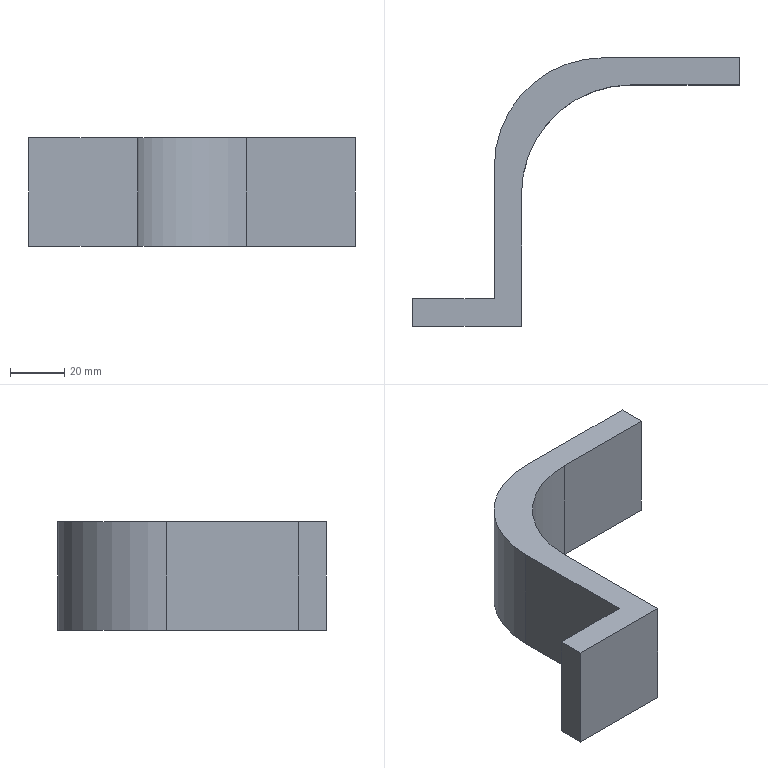Part | STEP file | Pressure Rod | 1 solid | 12 faces | box 120 x 98.5 x 40 mm | volume 83400 mm3 | plane 10 | cylinder 2 | commonest cylinder face diameters 80 x2
STEP:
#1=CARTESIAN_POINT('',(0.,0.,0.));
#2=DIRECTION('',(0.,0.,1.));
#3=DIRECTION('',(1.,0.,0.));
#4=AXIS2_PLACEMENT_3D('',#1,#2,#3);
#5=CARTESIAN_POINT('',(0.,-10.,-20.));
#6=VERTEX_POINT('',#5);
#7=CARTESIAN_POINT('',(0.,0.,-20.));
#8=VERTEX_POINT('',#7);
#9=CARTESIAN_POINT('',(0.,-10.,-20.));
#10=DIRECTION('',(0.,1.,0.));
#11=VECTOR('',#10,1.);
#12=LINE('',#9,#11);
#13=CARTESIAN_POINT('',(0.,-10.,20.));
#14=DIRECTION('',(-1.,0.,0.));
#15=DIRECTION('',(0.,0.,1.));
#16=AXIS2_PLACEMENT_3D('',#13,#14,#15);
#17=PLANE('',#16);
#18=CARTESIAN_POINT('',(-40.,0.));
#19=DIRECTION('',(0.,1.));
#20=VECTOR('',#19,1.);
#21=LINE('',#18,#20);
#22=(GEOMETRIC_REPRESENTATION_CONTEXT(2)PARAMETRIC_REPRESENTATION_CONTEXT()REPRESENTATION_CONTEXT('',''));
#23=DEFINITIONAL_REPRESENTATION('',(#21),#22);
#24=PCURVE('',#17,#23);
#25=CARTESIAN_POINT('',(0.,0.,-20.));
#26=DIRECTION('',(0.,0.,1.));
#27=DIRECTION('',(1.,0.,0.));
#28=AXIS2_PLACEMENT_3D('',#25,#26,#27);
#29=PLANE('',#28);
#30=CARTESIAN_POINT('',(0.,-10.));
#31=DIRECTION('',(0.,1.));
#32=VECTOR('',#31,1.);
#33=LINE('',#30,#32);
#34=(GEOMETRIC_REPRESENTATION_CONTEXT(2)PARAMETRIC_REPRESENTATION_CONTEXT()REPRESENTATION_CONTEXT('',''));
#35=DEFINITIONAL_REPRESENTATION('',(#33),#34);
#36=PCURVE('',#29,#35);
#37=SURFACE_CURVE('',#12,(#24,#36),.PCURVE_S1.);
#38=EDGE_CURVE('',#6,#8,#37,.T.);
#39=ORIENTED_EDGE('',*,*,#38,.T.);
#40=CARTESIAN_POINT('',(0.,0.,20.));
#41=VERTEX_POINT('',#40);
#42=CARTESIAN_POINT('',(0.,0.,20.));
#43=DIRECTION('',(0.,0.,-1.));
#44=VECTOR('',#43,1.);
#45=LINE('',#42,#44);
#46=CARTESIAN_POINT('',(0.,10.));
#47=DIRECTION('',(-1.,0.));
#48=VECTOR('',#47,1.);
#49=LINE('',#46,#48);
#50=(GEOMETRIC_REPRESENTATION_CONTEXT(2)PARAMETRIC_REPRESENTATION_CONTEXT()REPRESENTATION_CONTEXT('',''));
#51=DEFINITIONAL_REPRESENTATION('',(#49),#50);
#52=PCURVE('',#17,#51);
#53=CARTESIAN_POINT('',(0.,0.,20.));
#54=DIRECTION('',(0.,-1.,0.));
#55=DIRECTION('',(1.,0.,0.));
#56=AXIS2_PLACEMENT_3D('',#53,#54,#55);
#57=PLANE('',#56);
#58=CARTESIAN_POINT('',(0.,0.));
#59=DIRECTION('',(0.,-1.));
#60=VECTOR('',#59,1.);
#61=LINE('',#58,#60);
#62=(GEOMETRIC_REPRESENTATION_CONTEXT(2)PARAMETRIC_REPRESENTATION_CONTEXT()REPRESENTATION_CONTEXT('',''));
#63=DEFINITIONAL_REPRESENTATION('',(#61),#62);
#64=PCURVE('',#57,#63);
#65=SURFACE_CURVE('',#45,(#52,#64),.PCURVE_S1.);
#66=EDGE_CURVE('',#41,#8,#65,.T.);
#67=ORIENTED_EDGE('',*,*,#66,.F.);
#68=CARTESIAN_POINT('',(0.,-10.,20.));
#69=VERTEX_POINT('',#68);
#70=CARTESIAN_POINT('',(0.,-10.,20.));
#71=DIRECTION('',(0.,1.,0.));
#72=VECTOR('',#71,1.);
#73=LINE('',#70,#72);
#74=CARTESIAN_POINT('',(0.,0.));
#75=DIRECTION('',(0.,1.));
#76=VECTOR('',#75,1.);
#77=LINE('',#74,#76);
#78=(GEOMETRIC_REPRESENTATION_CONTEXT(2)PARAMETRIC_REPRESENTATION_CONTEXT()REPRESENTATION_CONTEXT('',''));
#79=DEFINITIONAL_REPRESENTATION('',(#77),#78);
#80=PCURVE('',#17,#79);
#81=CARTESIAN_POINT('',(0.,0.,20.));
#82=DIRECTION('',(0.,0.,1.));
#83=DIRECTION('',(1.,0.,0.));
#84=AXIS2_PLACEMENT_3D('',#81,#82,#83);
#85=PLANE('',#84);
#86=CARTESIAN_POINT('',(0.,-10.));
#87=DIRECTION('',(0.,1.));
#88=VECTOR('',#87,1.);
#89=LINE('',#86,#88);
#90=(GEOMETRIC_REPRESENTATION_CONTEXT(2)PARAMETRIC_REPRESENTATION_CONTEXT()REPRESENTATION_CONTEXT('',''));
#91=DEFINITIONAL_REPRESENTATION('',(#89),#90);
#92=PCURVE('',#85,#91);
#93=SURFACE_CURVE('',#73,(#80,#92),.PCURVE_S1.);
#94=EDGE_CURVE('',#69,#41,#93,.T.);
#95=ORIENTED_EDGE('',*,*,#94,.F.);
#96=CARTESIAN_POINT('',(0.,-10.,20.));
#97=DIRECTION('',(0.,0.,-1.));
#98=VECTOR('',#97,1.);
#99=LINE('',#96,#98);
#100=CARTESIAN_POINT('',(0.,0.));
#101=DIRECTION('',(-1.,0.));
#102=VECTOR('',#101,1.);
#103=LINE('',#100,#102);
#104=(GEOMETRIC_REPRESENTATION_CONTEXT(2)PARAMETRIC_REPRESENTATION_CONTEXT()REPRESENTATION_CONTEXT('',''));
#105=DEFINITIONAL_REPRESENTATION('',(#103),#104);
#106=PCURVE('',#17,#105);
#107=CARTESIAN_POINT('',(-80.,-10.,20.));
#108=DIRECTION('',(0.,1.,0.));
#109=DIRECTION('',(0.,0.,1.));
#110=AXIS2_PLACEMENT_3D('',#107,#108,#109);
#111=PLANE('',#110);
#112=CARTESIAN_POINT('',(0.,80.));
#113=DIRECTION('',(-1.,0.));
#114=VECTOR('',#113,1.);
#115=LINE('',#112,#114);
#116=(GEOMETRIC_REPRESENTATION_CONTEXT(2)PARAMETRIC_REPRESENTATION_CONTEXT()REPRESENTATION_CONTEXT('',''));
#117=DEFINITIONAL_REPRESENTATION('',(#115),#116);
#118=PCURVE('',#111,#117);
#119=SURFACE_CURVE('',#99,(#106,#118),.PCURVE_S1.);
#120=EDGE_CURVE('',#69,#6,#119,.T.);
#121=ORIENTED_EDGE('',*,*,#120,.T.);
#122=EDGE_LOOP('',(#39,#67,#95,#121));
#123=FACE_BOUND('',#122,.T.);
#124=ADVANCED_FACE('',(#123),#17,.F.);
#125=CARTESIAN_POINT('',(-50.,0.,-20.));
#126=VERTEX_POINT('',#125);
#127=CARTESIAN_POINT('',(0.,0.,-20.));
#128=DIRECTION('',(-1.,0.,0.));
#129=VECTOR('',#128,1.);
#130=LINE('',#127,#129);
#131=CARTESIAN_POINT('',(0.,-40.));
#132=DIRECTION('',(-1.,0.));
#133=VECTOR('',#132,1.);
#134=LINE('',#131,#133);
#135=(GEOMETRIC_REPRESENTATION_CONTEXT(2)PARAMETRIC_REPRESENTATION_CONTEXT()REPRESENTATION_CONTEXT('',''));
#136=DEFINITIONAL_REPRESENTATION('',(#134),#135);
#137=PCURVE('',#57,#136);
#138=CARTESIAN_POINT('',(0.,0.));
#139=DIRECTION('',(-1.,0.));
#140=VECTOR('',#139,1.);
#141=LINE('',#138,#140);
#142=(GEOMETRIC_REPRESENTATION_CONTEXT(2)PARAMETRIC_REPRESENTATION_CONTEXT()REPRESENTATION_CONTEXT('',''));
#143=DEFINITIONAL_REPRESENTATION('',(#141),#142);
#144=PCURVE('',#29,#143);
#145=SURFACE_CURVE('',#130,(#137,#144),.PCURVE_S1.);
#146=EDGE_CURVE('',#8,#126,#145,.T.);
#147=ORIENTED_EDGE('',*,*,#146,.T.);
#148=CARTESIAN_POINT('',(-50.,0.,20.));
#149=VERTEX_POINT('',#148);
#150=CARTESIAN_POINT('',(-50.,0.,20.));
#151=DIRECTION('',(0.,0.,1.));
#152=VECTOR('',#151,1.);
#153=LINE('',#150,#152);
#154=CARTESIAN_POINT('',(-50.,0.));
#155=DIRECTION('',(0.,1.));
#156=VECTOR('',#155,1.);
#157=LINE('',#154,#156);
#158=(GEOMETRIC_REPRESENTATION_CONTEXT(2)PARAMETRIC_REPRESENTATION_CONTEXT()REPRESENTATION_CONTEXT('',''));
#159=DEFINITIONAL_REPRESENTATION('',(#157),#158);
#160=PCURVE('',#57,#159);
#161=CARTESIAN_POINT('',(-50.,-40.,20.));
#162=DIRECTION('',(0.,0.,-1.));
#163=DIRECTION('',(-1.,0.,0.));
#164=AXIS2_PLACEMENT_3D('',#161,#162,#163);
#165=CYLINDRICAL_SURFACE('',#164,40.);
#166=CARTESIAN_POINT('',(1.571,0.));
#167=DIRECTION('',(0.,-1.));
#168=VECTOR('',#167,1.);
#169=LINE('',#166,#168);
#170=(GEOMETRIC_REPRESENTATION_CONTEXT(2)PARAMETRIC_REPRESENTATION_CONTEXT()REPRESENTATION_CONTEXT('',''));
#171=DEFINITIONAL_REPRESENTATION('',(#169),#170);
#172=PCURVE('',#165,#171);
#173=SURFACE_CURVE('',#153,(#160,#172),.PCURVE_S1.);
#174=EDGE_CURVE('',#126,#149,#173,.T.);
#175=ORIENTED_EDGE('',*,*,#174,.T.);
#176=CARTESIAN_POINT('',(0.,0.,20.));
#177=DIRECTION('',(-1.,0.,0.));
#178=VECTOR('',#177,1.);
#179=LINE('',#176,#178);
#180=CARTESIAN_POINT('',(0.,0.));
#181=DIRECTION('',(-1.,0.));
#182=VECTOR('',#181,1.);
#183=LINE('',#180,#182);
#184=(GEOMETRIC_REPRESENTATION_CONTEXT(2)PARAMETRIC_REPRESENTATION_CONTEXT()REPRESENTATION_CONTEXT('',''));
#185=DEFINITIONAL_REPRESENTATION('',(#183),#184);
#186=PCURVE('',#57,#185);
#187=CARTESIAN_POINT('',(0.,0.));
#188=DIRECTION('',(-1.,0.));
#189=VECTOR('',#188,1.);
#190=LINE('',#187,#189);
#191=(GEOMETRIC_REPRESENTATION_CONTEXT(2)PARAMETRIC_REPRESENTATION_CONTEXT()REPRESENTATION_CONTEXT('',''));
#192=DEFINITIONAL_REPRESENTATION('',(#190),#191);
#193=PCURVE('',#85,#192);
#194=SURFACE_CURVE('',#179,(#186,#193),.PCURVE_S1.);
#195=EDGE_CURVE('',#41,#149,#194,.T.);
#196=ORIENTED_EDGE('',*,*,#195,.F.);
#197=ORIENTED_EDGE('',*,*,#66,.T.);
#198=EDGE_LOOP('',(#147,#175,#196,#197));
#199=FACE_BOUND('',#198,.T.);
#200=ADVANCED_FACE('',(#199),#57,.F.);
#201=CARTESIAN_POINT('',(-90.,-40.,20.));
#202=VERTEX_POINT('',#201);
#203=CARTESIAN_POINT('',(-90.,-88.5,20.));
#204=VERTEX_POINT('',#203);
#205=CARTESIAN_POINT('',(-90.,0.,20.));
#206=DIRECTION('',(0.,-1.,0.));
#207=VECTOR('',#206,1.);
#208=LINE('',#205,#207);
#209=CARTESIAN_POINT('',(-90.,0.,20.));
#210=DIRECTION('',(1.,0.,0.));
#211=DIRECTION('',(0.,1.,0.));
#212=AXIS2_PLACEMENT_3D('',#209,#210,#211);
#213=PLANE('',#212);
#214=CARTESIAN_POINT('',(0.,0.));
#215=DIRECTION('',(-1.,0.));
#216=VECTOR('',#215,1.);
#217=LINE('',#214,#216);
#218=(GEOMETRIC_REPRESENTATION_CONTEXT(2)PARAMETRIC_REPRESENTATION_CONTEXT()REPRESENTATION_CONTEXT('',''));
#219=DEFINITIONAL_REPRESENTATION('',(#217),#218);
#220=PCURVE('',#213,#219);
#221=CARTESIAN_POINT('',(-90.,0.));
#222=DIRECTION('',(0.,-1.));
#223=VECTOR('',#222,1.);
#224=LINE('',#221,#223);
#225=(GEOMETRIC_REPRESENTATION_CONTEXT(2)PARAMETRIC_REPRESENTATION_CONTEXT()REPRESENTATION_CONTEXT('',''));
#226=DEFINITIONAL_REPRESENTATION('',(#224),#225);
#227=PCURVE('',#85,#226);
#228=SURFACE_CURVE('',#208,(#220,#227),.PCURVE_S1.);
#229=EDGE_CURVE('',#202,#204,#228,.T.);
#230=ORIENTED_EDGE('',*,*,#229,.F.);
#231=CARTESIAN_POINT('',(-90.,-40.,-20.));
#232=VERTEX_POINT('',#231);
#233=CARTESIAN_POINT('',(-90.,-40.,20.));
#234=DIRECTION('',(0.,0.,-1.));
#235=VECTOR('',#234,1.);
#236=LINE('',#233,#235);
#237=CARTESIAN_POINT('',(-40.,0.));
#238=DIRECTION('',(0.,-1.));
#239=VECTOR('',#238,1.);
#240=LINE('',#237,#239);
#241=(GEOMETRIC_REPRESENTATION_CONTEXT(2)PARAMETRIC_REPRESENTATION_CONTEXT()REPRESENTATION_CONTEXT('',''));
#242=DEFINITIONAL_REPRESENTATION('',(#240),#241);
#243=PCURVE('',#213,#242);
#244=CARTESIAN_POINT('',(0.,0.));
#245=DIRECTION('',(0.,1.));
#246=VECTOR('',#245,1.);
#247=LINE('',#244,#246);
#248=(GEOMETRIC_REPRESENTATION_CONTEXT(2)PARAMETRIC_REPRESENTATION_CONTEXT()REPRESENTATION_CONTEXT('',''));
#249=DEFINITIONAL_REPRESENTATION('',(#247),#248);
#250=PCURVE('',#165,#249);
#251=SURFACE_CURVE('',#236,(#243,#250),.PCURVE_S1.);
#252=EDGE_CURVE('',#202,#232,#251,.T.);
#253=ORIENTED_EDGE('',*,*,#252,.T.);
#254=CARTESIAN_POINT('',(-90.,-88.5,-20.));
#255=VERTEX_POINT('',#254);
#256=CARTESIAN_POINT('',(-90.,0.,-20.));
#257=DIRECTION('',(0.,-1.,0.));
#258=VECTOR('',#257,1.);
#259=LINE('',#256,#258);
#260=CARTESIAN_POINT('',(0.,-40.));
#261=DIRECTION('',(-1.,0.));
#262=VECTOR('',#261,1.);
#263=LINE('',#260,#262);
#264=(GEOMETRIC_REPRESENTATION_CONTEXT(2)PARAMETRIC_REPRESENTATION_CONTEXT()REPRESENTATION_CONTEXT('',''));
#265=DEFINITIONAL_REPRESENTATION('',(#263),#264);
#266=PCURVE('',#213,#265);
#267=CARTESIAN_POINT('',(-90.,0.));
#268=DIRECTION('',(0.,-1.));
#269=VECTOR('',#268,1.);
#270=LINE('',#267,#269);
#271=(GEOMETRIC_REPRESENTATION_CONTEXT(2)PARAMETRIC_REPRESENTATION_CONTEXT()REPRESENTATION_CONTEXT('',''));
#272=DEFINITIONAL_REPRESENTATION('',(#270),#271);
#273=PCURVE('',#29,#272);
#274=SURFACE_CURVE('',#259,(#266,#273),.PCURVE_S1.);
#275=EDGE_CURVE('',#232,#255,#274,.T.);
#276=ORIENTED_EDGE('',*,*,#275,.T.);
#277=CARTESIAN_POINT('',(-90.,-88.5,20.));
#278=DIRECTION('',(0.,0.,-1.));
#279=VECTOR('',#278,1.);
#280=LINE('',#277,#279);
#281=CARTESIAN_POINT('',(-88.5,0.));
#282=DIRECTION('',(0.,-1.));
#283=VECTOR('',#282,1.);
#284=LINE('',#281,#283);
#285=(GEOMETRIC_REPRESENTATION_CONTEXT(2)PARAMETRIC_REPRESENTATION_CONTEXT()REPRESENTATION_CONTEXT('',''));
#286=DEFINITIONAL_REPRESENTATION('',(#284),#285);
#287=PCURVE('',#213,#286);
#288=CARTESIAN_POINT('',(-90.,-88.5,20.));
#289=DIRECTION('',(0.,-1.,0.));
#290=DIRECTION('',(0.,0.,-1.));
#291=AXIS2_PLACEMENT_3D('',#288,#289,#290);
#292=PLANE('',#291);
#293=CARTESIAN_POINT('',(0.,0.));
#294=DIRECTION('',(1.,0.));
#295=VECTOR('',#294,1.);
#296=LINE('',#293,#295);
#297=(GEOMETRIC_REPRESENTATION_CONTEXT(2)PARAMETRIC_REPRESENTATION_CONTEXT()REPRESENTATION_CONTEXT('',''));
#298=DEFINITIONAL_REPRESENTATION('',(#296),#297);
#299=PCURVE('',#292,#298);
#300=SURFACE_CURVE('',#280,(#287,#299),.PCURVE_S1.);
#301=EDGE_CURVE('',#204,#255,#300,.T.);
#302=ORIENTED_EDGE('',*,*,#301,.F.);
#303=EDGE_LOOP('',(#230,#253,#276,#302));
#304=FACE_BOUND('',#303,.T.);
#305=ADVANCED_FACE('',(#304),#213,.F.);
#306=CARTESIAN_POINT('',(-120.,-88.5,-20.));
#307=VERTEX_POINT('',#306);
#308=CARTESIAN_POINT('',(-90.,-88.5,-20.));
#309=DIRECTION('',(-1.,0.,0.));
#310=VECTOR('',#309,1.);
#311=LINE('',#308,#310);
#312=CARTESIAN_POINT('',(40.,0.));
#313=DIRECTION('',(0.,-1.));
#314=VECTOR('',#313,1.);
#315=LINE('',#312,#314);
#316=(GEOMETRIC_REPRESENTATION_CONTEXT(2)PARAMETRIC_REPRESENTATION_CONTEXT()REPRESENTATION_CONTEXT('',''));
#317=DEFINITIONAL_REPRESENTATION('',(#315),#316);
#318=PCURVE('',#292,#317);
#319=CARTESIAN_POINT('',(-90.,-88.5));
#320=DIRECTION('',(-1.,0.));
#321=VECTOR('',#320,1.);
#322=LINE('',#319,#321);
#323=(GEOMETRIC_REPRESENTATION_CONTEXT(2)PARAMETRIC_REPRESENTATION_CONTEXT()REPRESENTATION_CONTEXT('',''));
#324=DEFINITIONAL_REPRESENTATION('',(#322),#323);
#325=PCURVE('',#29,#324);
#326=SURFACE_CURVE('',#311,(#318,#325),.PCURVE_S1.);
#327=EDGE_CURVE('',#255,#307,#326,.T.);
#328=ORIENTED_EDGE('',*,*,#327,.T.);
#329=CARTESIAN_POINT('',(-120.,-88.5,20.));
#330=VERTEX_POINT('',#329);
#331=CARTESIAN_POINT('',(-120.,-88.5,20.));
#332=DIRECTION('',(0.,0.,-1.));
#333=VECTOR('',#332,1.);
#334=LINE('',#331,#333);
#335=CARTESIAN_POINT('',(0.,-30.));
#336=DIRECTION('',(1.,0.));
#337=VECTOR('',#336,1.);
#338=LINE('',#335,#337);
#339=(GEOMETRIC_REPRESENTATION_CONTEXT(2)PARAMETRIC_REPRESENTATION_CONTEXT()REPRESENTATION_CONTEXT('',''));
#340=DEFINITIONAL_REPRESENTATION('',(#338),#339);
#341=PCURVE('',#292,#340);
#342=CARTESIAN_POINT('',(-120.,-88.5,20.));
#343=DIRECTION('',(1.,0.,0.));
#344=DIRECTION('',(0.,1.,0.));
#345=AXIS2_PLACEMENT_3D('',#342,#343,#344);
#346=PLANE('',#345);
#347=CARTESIAN_POINT('',(0.,0.));
#348=DIRECTION('',(0.,-1.));
#349=VECTOR('',#348,1.);
#350=LINE('',#347,#349);
#351=(GEOMETRIC_REPRESENTATION_CONTEXT(2)PARAMETRIC_REPRESENTATION_CONTEXT()REPRESENTATION_CONTEXT('',''));
#352=DEFINITIONAL_REPRESENTATION('',(#350),#351);
#353=PCURVE('',#346,#352);
#354=SURFACE_CURVE('',#334,(#341,#353),.PCURVE_S1.);
#355=EDGE_CURVE('',#330,#307,#354,.T.);
#356=ORIENTED_EDGE('',*,*,#355,.F.);
#357=CARTESIAN_POINT('',(-90.,-88.5,20.));
#358=DIRECTION('',(-1.,0.,0.));
#359=VECTOR('',#358,1.);
#360=LINE('',#357,#359);
#361=CARTESIAN_POINT('',(0.,0.));
#362=DIRECTION('',(0.,-1.));
#363=VECTOR('',#362,1.);
#364=LINE('',#361,#363);
#365=(GEOMETRIC_REPRESENTATION_CONTEXT(2)PARAMETRIC_REPRESENTATION_CONTEXT()REPRESENTATION_CONTEXT('',''));
#366=DEFINITIONAL_REPRESENTATION('',(#364),#365);
#367=PCURVE('',#292,#366);
#368=CARTESIAN_POINT('',(-90.,-88.5));
#369=DIRECTION('',(-1.,0.));
#370=VECTOR('',#369,1.);
#371=LINE('',#368,#370);
#372=(GEOMETRIC_REPRESENTATION_CONTEXT(2)PARAMETRIC_REPRESENTATION_CONTEXT()REPRESENTATION_CONTEXT('',''));
#373=DEFINITIONAL_REPRESENTATION('',(#371),#372);
#374=PCURVE('',#85,#373);
#375=SURFACE_CURVE('',#360,(#367,#374),.PCURVE_S1.);
#376=EDGE_CURVE('',#204,#330,#375,.T.);
#377=ORIENTED_EDGE('',*,*,#376,.F.);
#378=ORIENTED_EDGE('',*,*,#301,.T.);
#379=EDGE_LOOP('',(#328,#356,#377,#378));
#380=FACE_BOUND('',#379,.T.);
#381=ADVANCED_FACE('',(#380),#292,.F.);
#382=CARTESIAN_POINT('',(-120.,-98.5,-20.));
#383=VERTEX_POINT('',#382);
#384=CARTESIAN_POINT('',(-120.,-88.5,-20.));
#385=DIRECTION('',(0.,-1.,0.));
#386=VECTOR('',#385,1.);
#387=LINE('',#384,#386);
#388=CARTESIAN_POINT('',(0.,-40.));
#389=DIRECTION('',(-1.,0.));
#390=VECTOR('',#389,1.);
#391=LINE('',#388,#390);
#392=(GEOMETRIC_REPRESENTATION_CONTEXT(2)PARAMETRIC_REPRESENTATION_CONTEXT()REPRESENTATION_CONTEXT('',''));
#393=DEFINITIONAL_REPRESENTATION('',(#391),#392);
#394=PCURVE('',#346,#393);
#395=CARTESIAN_POINT('',(-120.,-88.5));
#396=DIRECTION('',(0.,-1.));
#397=VECTOR('',#396,1.);
#398=LINE('',#395,#397);
#399=(GEOMETRIC_REPRESENTATION_CONTEXT(2)PARAMETRIC_REPRESENTATION_CONTEXT()REPRESENTATION_CONTEXT('',''));
#400=DEFINITIONAL_REPRESENTATION('',(#398),#399);
#401=PCURVE('',#29,#400);
#402=SURFACE_CURVE('',#387,(#394,#401),.PCURVE_S1.);
#403=EDGE_CURVE('',#307,#383,#402,.T.);
#404=ORIENTED_EDGE('',*,*,#403,.T.);
#405=CARTESIAN_POINT('',(-120.,-98.5,20.));
#406=VERTEX_POINT('',#405);
#407=CARTESIAN_POINT('',(-120.,-98.5,20.));
#408=DIRECTION('',(0.,0.,-1.));
#409=VECTOR('',#408,1.);
#410=LINE('',#407,#409);
#411=CARTESIAN_POINT('',(-10.,0.));
#412=DIRECTION('',(0.,-1.));
#413=VECTOR('',#412,1.);
#414=LINE('',#411,#413);
#415=(GEOMETRIC_REPRESENTATION_CONTEXT(2)PARAMETRIC_REPRESENTATION_CONTEXT()REPRESENTATION_CONTEXT('',''));
#416=DEFINITIONAL_REPRESENTATION('',(#414),#415);
#417=PCURVE('',#346,#416);
#418=CARTESIAN_POINT('',(-120.,-98.5,20.));
#419=DIRECTION('',(0.,1.,0.));
#420=DIRECTION('',(0.,0.,1.));
#421=AXIS2_PLACEMENT_3D('',#418,#419,#420);
#422=PLANE('',#421);
#423=CARTESIAN_POINT('',(0.,0.));
#424=DIRECTION('',(-1.,0.));
#425=VECTOR('',#424,1.);
#426=LINE('',#423,#425);
#427=(GEOMETRIC_REPRESENTATION_CONTEXT(2)PARAMETRIC_REPRESENTATION_CONTEXT()REPRESENTATION_CONTEXT('',''));
#428=DEFINITIONAL_REPRESENTATION('',(#426),#427);
#429=PCURVE('',#422,#428);
#430=SURFACE_CURVE('',#410,(#417,#429),.PCURVE_S1.);
#431=EDGE_CURVE('',#406,#383,#430,.T.);
#432=ORIENTED_EDGE('',*,*,#431,.F.);
#433=CARTESIAN_POINT('',(-120.,-88.5,20.));
#434=DIRECTION('',(0.,-1.,0.));
#435=VECTOR('',#434,1.);
#436=LINE('',#433,#435);
#437=CARTESIAN_POINT('',(0.,0.));
#438=DIRECTION('',(-1.,0.));
#439=VECTOR('',#438,1.);
#440=LINE('',#437,#439);
#441=(GEOMETRIC_REPRESENTATION_CONTEXT(2)PARAMETRIC_REPRESENTATION_CONTEXT()REPRESENTATION_CONTEXT('',''));
#442=DEFINITIONAL_REPRESENTATION('',(#440),#441);
#443=PCURVE('',#346,#442);
#444=CARTESIAN_POINT('',(-120.,-88.5));
#445=DIRECTION('',(0.,-1.));
#446=VECTOR('',#445,1.);
#447=LINE('',#444,#446);
#448=(GEOMETRIC_REPRESENTATION_CONTEXT(2)PARAMETRIC_REPRESENTATION_CONTEXT()REPRESENTATION_CONTEXT('',''));
#449=DEFINITIONAL_REPRESENTATION('',(#447),#448);
#450=PCURVE('',#85,#449);
#451=SURFACE_CURVE('',#436,(#443,#450),.PCURVE_S1.);
#452=EDGE_CURVE('',#330,#406,#451,.T.);
#453=ORIENTED_EDGE('',*,*,#452,.F.);
#454=ORIENTED_EDGE('',*,*,#355,.T.);
#455=EDGE_LOOP('',(#404,#432,#453,#454));
#456=FACE_BOUND('',#455,.T.);
#457=ADVANCED_FACE('',(#456),#346,.F.);
#458=CARTESIAN_POINT('',(-80.,-98.5,-20.));
#459=VERTEX_POINT('',#458);
#460=CARTESIAN_POINT('',(-120.,-98.5,-20.));
#461=DIRECTION('',(1.,0.,0.));
#462=VECTOR('',#461,1.);
#463=LINE('',#460,#462);
#464=CARTESIAN_POINT('',(-40.,0.));
#465=DIRECTION('',(0.,1.));
#466=VECTOR('',#465,1.);
#467=LINE('',#464,#466);
#468=(GEOMETRIC_REPRESENTATION_CONTEXT(2)PARAMETRIC_REPRESENTATION_CONTEXT()REPRESENTATION_CONTEXT('',''));
#469=DEFINITIONAL_REPRESENTATION('',(#467),#468);
#470=PCURVE('',#422,#469);
#471=CARTESIAN_POINT('',(-120.,-98.5));
#472=DIRECTION('',(1.,0.));
#473=VECTOR('',#472,1.);
#474=LINE('',#471,#473);
#475=(GEOMETRIC_REPRESENTATION_CONTEXT(2)PARAMETRIC_REPRESENTATION_CONTEXT()REPRESENTATION_CONTEXT('',''));
#476=DEFINITIONAL_REPRESENTATION('',(#474),#475);
#477=PCURVE('',#29,#476);
#478=SURFACE_CURVE('',#463,(#470,#477),.PCURVE_S1.);
#479=EDGE_CURVE('',#383,#459,#478,.T.);
#480=ORIENTED_EDGE('',*,*,#479,.T.);
#481=CARTESIAN_POINT('',(-80.,-98.5,20.));
#482=VERTEX_POINT('',#481);
#483=CARTESIAN_POINT('',(-80.,-98.5,20.));
#484=DIRECTION('',(0.,0.,-1.));
#485=VECTOR('',#484,1.);
#486=LINE('',#483,#485);
#487=CARTESIAN_POINT('',(0.,40.));
#488=DIRECTION('',(-1.,0.));
#489=VECTOR('',#488,1.);
#490=LINE('',#487,#489);
#491=(GEOMETRIC_REPRESENTATION_CONTEXT(2)PARAMETRIC_REPRESENTATION_CONTEXT()REPRESENTATION_CONTEXT('',''));
#492=DEFINITIONAL_REPRESENTATION('',(#490),#491);
#493=PCURVE('',#422,#492);
#494=CARTESIAN_POINT('',(-80.,-98.5,20.));
#495=DIRECTION('',(-1.,0.,0.));
#496=DIRECTION('',(0.,0.,1.));
#497=AXIS2_PLACEMENT_3D('',#494,#495,#496);
#498=PLANE('',#497);
#499=CARTESIAN_POINT('',(0.,0.));
#500=DIRECTION('',(-1.,0.));
#501=VECTOR('',#500,1.);
#502=LINE('',#499,#501);
#503=(GEOMETRIC_REPRESENTATION_CONTEXT(2)PARAMETRIC_REPRESENTATION_CONTEXT()REPRESENTATION_CONTEXT('',''));
#504=DEFINITIONAL_REPRESENTATION('',(#502),#503);
#505=PCURVE('',#498,#504);
#506=SURFACE_CURVE('',#486,(#493,#505),.PCURVE_S1.);
#507=EDGE_CURVE('',#482,#459,#506,.T.);
#508=ORIENTED_EDGE('',*,*,#507,.F.);
#509=CARTESIAN_POINT('',(-120.,-98.5,20.));
#510=DIRECTION('',(1.,0.,0.));
#511=VECTOR('',#510,1.);
#512=LINE('',#509,#511);
#513=CARTESIAN_POINT('',(0.,0.));
#514=DIRECTION('',(0.,1.));
#515=VECTOR('',#514,1.);
#516=LINE('',#513,#515);
#517=(GEOMETRIC_REPRESENTATION_CONTEXT(2)PARAMETRIC_REPRESENTATION_CONTEXT()REPRESENTATION_CONTEXT('',''));
#518=DEFINITIONAL_REPRESENTATION('',(#516),#517);
#519=PCURVE('',#422,#518);
#520=CARTESIAN_POINT('',(-120.,-98.5));
#521=DIRECTION('',(1.,0.));
#522=VECTOR('',#521,1.);
#523=LINE('',#520,#522);
#524=(GEOMETRIC_REPRESENTATION_CONTEXT(2)PARAMETRIC_REPRESENTATION_CONTEXT()REPRESENTATION_CONTEXT('',''));
#525=DEFINITIONAL_REPRESENTATION('',(#523),#524);
#526=PCURVE('',#85,#525);
#527=SURFACE_CURVE('',#512,(#519,#526),.PCURVE_S1.);
#528=EDGE_CURVE('',#406,#482,#527,.T.);
#529=ORIENTED_EDGE('',*,*,#528,.F.);
#530=ORIENTED_EDGE('',*,*,#431,.T.);
#531=EDGE_LOOP('',(#480,#508,#529,#530));
#532=FACE_BOUND('',#531,.T.);
#533=ADVANCED_FACE('',(#532),#422,.F.);
#534=CARTESIAN_POINT('',(-80.,-50.,-20.));
#535=VERTEX_POINT('',#534);
#536=CARTESIAN_POINT('',(-80.,-98.5,-20.));
#537=DIRECTION('',(0.,1.,0.));
#538=VECTOR('',#537,1.);
#539=LINE('',#536,#538);
#540=CARTESIAN_POINT('',(-40.,0.));
#541=DIRECTION('',(0.,1.));
#542=VECTOR('',#541,1.);
#543=LINE('',#540,#542);
#544=(GEOMETRIC_REPRESENTATION_CONTEXT(2)PARAMETRIC_REPRESENTATION_CONTEXT()REPRESENTATION_CONTEXT('',''));
#545=DEFINITIONAL_REPRESENTATION('',(#543),#544);
#546=PCURVE('',#498,#545);
#547=CARTESIAN_POINT('',(-80.,-98.5));
#548=DIRECTION('',(0.,1.));
#549=VECTOR('',#548,1.);
#550=LINE('',#547,#549);
#551=(GEOMETRIC_REPRESENTATION_CONTEXT(2)PARAMETRIC_REPRESENTATION_CONTEXT()REPRESENTATION_CONTEXT('',''));
#552=DEFINITIONAL_REPRESENTATION('',(#550),#551);
#553=PCURVE('',#29,#552);
#554=SURFACE_CURVE('',#539,(#546,#553),.PCURVE_S1.);
#555=EDGE_CURVE('',#459,#535,#554,.T.);
#556=ORIENTED_EDGE('',*,*,#555,.T.);
#557=CARTESIAN_POINT('',(-80.,-50.,20.));
#558=VERTEX_POINT('',#557);
#559=CARTESIAN_POINT('',(-80.,-50.,20.));
#560=DIRECTION('',(0.,0.,1.));
#561=VECTOR('',#560,1.);
#562=LINE('',#559,#561);
#563=CARTESIAN_POINT('',(0.,48.5));
#564=DIRECTION('',(1.,0.));
#565=VECTOR('',#564,1.);
#566=LINE('',#563,#565);
#567=(GEOMETRIC_REPRESENTATION_CONTEXT(2)PARAMETRIC_REPRESENTATION_CONTEXT()REPRESENTATION_CONTEXT('',''));
#568=DEFINITIONAL_REPRESENTATION('',(#566),#567);
#569=PCURVE('',#498,#568);
#570=CARTESIAN_POINT('',(-40.,-50.,20.));
#571=DIRECTION('',(0.,0.,1.));
#572=DIRECTION('',(1.,0.,0.));
#573=AXIS2_PLACEMENT_3D('',#570,#571,#572);
#574=CYLINDRICAL_SURFACE('',#573,40.);
#575=CARTESIAN_POINT('',(3.142,0.));
#576=DIRECTION('',(0.,1.));
#577=VECTOR('',#576,1.);
#578=LINE('',#575,#577);
#579=(GEOMETRIC_REPRESENTATION_CONTEXT(2)PARAMETRIC_REPRESENTATION_CONTEXT()REPRESENTATION_CONTEXT('',''));
#580=DEFINITIONAL_REPRESENTATION('',(#578),#579);
#581=PCURVE('',#574,#580);
#582=SURFACE_CURVE('',#562,(#569,#581),.PCURVE_S1.);
#583=EDGE_CURVE('',#535,#558,#582,.T.);
#584=ORIENTED_EDGE('',*,*,#583,.T.);
#585=CARTESIAN_POINT('',(-80.,-98.5,20.));
#586=DIRECTION('',(0.,1.,0.));
#587=VECTOR('',#586,1.);
#588=LINE('',#585,#587);
#589=CARTESIAN_POINT('',(0.,0.));
#590=DIRECTION('',(0.,1.));
#591=VECTOR('',#590,1.);
#592=LINE('',#589,#591);
#593=(GEOMETRIC_REPRESENTATION_CONTEXT(2)PARAMETRIC_REPRESENTATION_CONTEXT()REPRESENTATION_CONTEXT('',''));
#594=DEFINITIONAL_REPRESENTATION('',(#592),#593);
#595=PCURVE('',#498,#594);
#596=CARTESIAN_POINT('',(-80.,-98.5));
#597=DIRECTION('',(0.,1.));
#598=VECTOR('',#597,1.);
#599=LINE('',#596,#598);
#600=(GEOMETRIC_REPRESENTATION_CONTEXT(2)PARAMETRIC_REPRESENTATION_CONTEXT()REPRESENTATION_CONTEXT('',''));
#601=DEFINITIONAL_REPRESENTATION('',(#599),#600);
#602=PCURVE('',#85,#601);
#603=SURFACE_CURVE('',#588,(#595,#602),.PCURVE_S1.);
#604=EDGE_CURVE('',#482,#558,#603,.T.);
#605=ORIENTED_EDGE('',*,*,#604,.F.);
#606=ORIENTED_EDGE('',*,*,#507,.T.);
#607=EDGE_LOOP('',(#556,#584,#605,#606));
#608=FACE_BOUND('',#607,.T.);
#609=ADVANCED_FACE('',(#608),#498,.F.);
#610=CARTESIAN_POINT('',(-40.,-10.,20.));
#611=VERTEX_POINT('',#610);
#612=CARTESIAN_POINT('',(-80.,-10.,20.));
#613=DIRECTION('',(1.,0.,0.));
#614=VECTOR('',#613,1.);
#615=LINE('',#612,#614);
#616=CARTESIAN_POINT('',(0.,0.));
#617=DIRECTION('',(0.,1.));
#618=VECTOR('',#617,1.);
#619=LINE('',#616,#618);
#620=(GEOMETRIC_REPRESENTATION_CONTEXT(2)PARAMETRIC_REPRESENTATION_CONTEXT()REPRESENTATION_CONTEXT('',''));
#621=DEFINITIONAL_REPRESENTATION('',(#619),#620);
#622=PCURVE('',#111,#621);
#623=CARTESIAN_POINT('',(-80.,-10.));
#624=DIRECTION('',(1.,0.));
#625=VECTOR('',#624,1.);
#626=LINE('',#623,#625);
#627=(GEOMETRIC_REPRESENTATION_CONTEXT(2)PARAMETRIC_REPRESENTATION_CONTEXT()REPRESENTATION_CONTEXT('',''));
#628=DEFINITIONAL_REPRESENTATION('',(#626),#627);
#629=PCURVE('',#85,#628);
#630=SURFACE_CURVE('',#615,(#622,#629),.PCURVE_S1.);
#631=EDGE_CURVE('',#611,#69,#630,.T.);
#632=ORIENTED_EDGE('',*,*,#631,.F.);
#633=CARTESIAN_POINT('',(-40.,-10.,-20.));
#634=VERTEX_POINT('',#633);
#635=CARTESIAN_POINT('',(-40.,-10.,-20.));
#636=DIRECTION('',(0.,0.,-1.));
#637=VECTOR('',#636,1.);
#638=LINE('',#635,#637);
#639=CARTESIAN_POINT('',(-40.,40.));
#640=DIRECTION('',(-1.,0.));
#641=VECTOR('',#640,1.);
#642=LINE('',#639,#641);
#643=(GEOMETRIC_REPRESENTATION_CONTEXT(2)PARAMETRIC_REPRESENTATION_CONTEXT()REPRESENTATION_CONTEXT('',''));
#644=DEFINITIONAL_REPRESENTATION('',(#642),#643);
#645=PCURVE('',#111,#644);
#646=CARTESIAN_POINT('',(1.571,-40.));
#647=DIRECTION('',(0.,-1.));
#648=VECTOR('',#647,1.);
#649=LINE('',#646,#648);
#650=(GEOMETRIC_REPRESENTATION_CONTEXT(2)PARAMETRIC_REPRESENTATION_CONTEXT()REPRESENTATION_CONTEXT('',''));
#651=DEFINITIONAL_REPRESENTATION('',(#649),#650);
#652=PCURVE('',#574,#651);
#653=SURFACE_CURVE('',#638,(#645,#652),.PCURVE_S1.);
#654=EDGE_CURVE('',#611,#634,#653,.T.);
#655=ORIENTED_EDGE('',*,*,#654,.T.);
#656=CARTESIAN_POINT('',(-80.,-10.,-20.));
#657=DIRECTION('',(1.,0.,0.));
#658=VECTOR('',#657,1.);
#659=LINE('',#656,#658);
#660=CARTESIAN_POINT('',(-40.,0.));
#661=DIRECTION('',(0.,1.));
#662=VECTOR('',#661,1.);
#663=LINE('',#660,#662);
#664=(GEOMETRIC_REPRESENTATION_CONTEXT(2)PARAMETRIC_REPRESENTATION_CONTEXT()REPRESENTATION_CONTEXT('',''));
#665=DEFINITIONAL_REPRESENTATION('',(#663),#664);
#666=PCURVE('',#111,#665);
#667=CARTESIAN_POINT('',(-80.,-10.));
#668=DIRECTION('',(1.,0.));
#669=VECTOR('',#668,1.);
#670=LINE('',#667,#669);
#671=(GEOMETRIC_REPRESENTATION_CONTEXT(2)PARAMETRIC_REPRESENTATION_CONTEXT()REPRESENTATION_CONTEXT('',''));
#672=DEFINITIONAL_REPRESENTATION('',(#670),#671);
#673=PCURVE('',#29,#672);
#674=SURFACE_CURVE('',#659,(#666,#673),.PCURVE_S1.);
#675=EDGE_CURVE('',#634,#6,#674,.T.);
#676=ORIENTED_EDGE('',*,*,#675,.T.);
#677=ORIENTED_EDGE('',*,*,#120,.F.);
#678=EDGE_LOOP('',(#632,#655,#676,#677));
#679=FACE_BOUND('',#678,.T.);
#680=ADVANCED_FACE('',(#679),#111,.F.);
#681=ORIENTED_EDGE('',*,*,#195,.T.);
#682=CARTESIAN_POINT('',(-50.,-40.,20.));
#683=DIRECTION('',(0.,0.,1.));
#684=DIRECTION('',(1.,0.,0.));
#685=AXIS2_PLACEMENT_3D('',#682,#683,#684);
#686=CIRCLE('',#685,40.);
#687=CARTESIAN_POINT('',(-50.,-40.));
#688=DIRECTION('',(1.,0.));
#689=AXIS2_PLACEMENT_2D('',#687,#688);
#690=CIRCLE('',#689,40.);
#691=(GEOMETRIC_REPRESENTATION_CONTEXT(2)PARAMETRIC_REPRESENTATION_CONTEXT()REPRESENTATION_CONTEXT('',''));
#692=DEFINITIONAL_REPRESENTATION('',(#690),#691);
#693=PCURVE('',#85,#692);
#694=CARTESIAN_POINT('',(3.142,0.));
#695=DIRECTION('',(-1.,0.));
#696=VECTOR('',#695,1.);
#697=LINE('',#694,#696);
#698=(GEOMETRIC_REPRESENTATION_CONTEXT(2)PARAMETRIC_REPRESENTATION_CONTEXT()REPRESENTATION_CONTEXT('',''));
#699=DEFINITIONAL_REPRESENTATION('',(#697),#698);
#700=PCURVE('',#165,#699);
#701=SURFACE_CURVE('',#686,(#693,#700),.PCURVE_S1.);
#702=EDGE_CURVE('',#149,#202,#701,.T.);
#703=ORIENTED_EDGE('',*,*,#702,.T.);
#704=ORIENTED_EDGE('',*,*,#229,.T.);
#705=ORIENTED_EDGE('',*,*,#376,.T.);
#706=ORIENTED_EDGE('',*,*,#452,.T.);
#707=ORIENTED_EDGE('',*,*,#528,.T.);
#708=ORIENTED_EDGE('',*,*,#604,.T.);
#709=CARTESIAN_POINT('',(-40.,-50.,20.));
#710=DIRECTION('',(0.,0.,-1.));
#711=DIRECTION('',(1.,0.,0.));
#712=AXIS2_PLACEMENT_3D('',#709,#710,#711);
#713=CIRCLE('',#712,40.);
#714=CARTESIAN_POINT('',(0.,-50.));
#715=CARTESIAN_POINT('',(0.,-119.282));
#716=CARTESIAN_POINT('',(-60.,-84.641));
#717=CARTESIAN_POINT('',(-120.,-50.));
#718=CARTESIAN_POINT('',(-60.,-15.359));
#719=CARTESIAN_POINT('',(0.,19.282));
#720=CARTESIAN_POINT('',(0.,-50.));
#721=(BOUNDED_CURVE()B_SPLINE_CURVE(2,(#714,#715,#716,#717,#718,#719,#720),.UNSPECIFIED.,.T.,.F.)B_SPLINE_CURVE_WITH_KNOTS((1,2,2,2,2,1),(-2.094,0.,2.094,4.189,6.283,8.378),.UNSPECIFIED.)CURVE()GEOMETRIC_REPRESENTATION_ITEM()RATIONAL_B_SPLINE_CURVE((1.,0.5,1.,0.5,1.,0.5,1.))REPRESENTATION_ITEM(''));
#722=(GEOMETRIC_REPRESENTATION_CONTEXT(2)PARAMETRIC_REPRESENTATION_CONTEXT()REPRESENTATION_CONTEXT('',''));
#723=DEFINITIONAL_REPRESENTATION('',(#721),#722);
#724=PCURVE('',#85,#723);
#725=CARTESIAN_POINT('',(6.283,0.));
#726=DIRECTION('',(-1.,0.));
#727=VECTOR('',#726,1.);
#728=LINE('',#725,#727);
#729=(GEOMETRIC_REPRESENTATION_CONTEXT(2)PARAMETRIC_REPRESENTATION_CONTEXT()REPRESENTATION_CONTEXT('',''));
#730=DEFINITIONAL_REPRESENTATION('',(#728),#729);
#731=PCURVE('',#574,#730);
#732=SURFACE_CURVE('',#713,(#724,#731),.PCURVE_S1.);
#733=EDGE_CURVE('',#558,#611,#732,.T.);
#734=ORIENTED_EDGE('',*,*,#733,.T.);
#735=ORIENTED_EDGE('',*,*,#631,.T.);
#736=ORIENTED_EDGE('',*,*,#94,.T.);
#737=EDGE_LOOP('',(#681,#703,#704,#705,#706,#707,#708,#734,#735,#736));
#738=FACE_BOUND('',#737,.T.);
#739=ADVANCED_FACE('',(#738),#85,.T.);
#740=ORIENTED_EDGE('',*,*,#275,.F.);
#741=CARTESIAN_POINT('',(-50.,-40.,-20.));
#742=DIRECTION('',(0.,0.,-1.));
#743=DIRECTION('',(1.,0.,0.));
#744=AXIS2_PLACEMENT_3D('',#741,#742,#743);
#745=CIRCLE('',#744,40.);
#746=CARTESIAN_POINT('',(-10.,-40.));
#747=CARTESIAN_POINT('',(-10.,-109.282));
#748=CARTESIAN_POINT('',(-70.,-74.641));
#749=CARTESIAN_POINT('',(-130.,-40.));
#750=CARTESIAN_POINT('',(-70.,-5.359));
#751=CARTESIAN_POINT('',(-10.,29.282));
#752=CARTESIAN_POINT('',(-10.,-40.));
#753=(BOUNDED_CURVE()B_SPLINE_CURVE(2,(#746,#747,#748,#749,#750,#751,#752),.UNSPECIFIED.,.T.,.F.)B_SPLINE_CURVE_WITH_KNOTS((1,2,2,2,2,1),(-2.094,0.,2.094,4.189,6.283,8.378),.UNSPECIFIED.)CURVE()GEOMETRIC_REPRESENTATION_ITEM()RATIONAL_B_SPLINE_CURVE((1.,0.5,1.,0.5,1.,0.5,1.))REPRESENTATION_ITEM(''));
#754=(GEOMETRIC_REPRESENTATION_CONTEXT(2)PARAMETRIC_REPRESENTATION_CONTEXT()REPRESENTATION_CONTEXT('',''));
#755=DEFINITIONAL_REPRESENTATION('',(#753),#754);
#756=PCURVE('',#29,#755);
#757=CARTESIAN_POINT('',(-3.142,40.));
#758=DIRECTION('',(1.,0.));
#759=VECTOR('',#758,1.);
#760=LINE('',#757,#759);
#761=(GEOMETRIC_REPRESENTATION_CONTEXT(2)PARAMETRIC_REPRESENTATION_CONTEXT()REPRESENTATION_CONTEXT('',''));
#762=DEFINITIONAL_REPRESENTATION('',(#760),#761);
#763=PCURVE('',#165,#762);
#764=SURFACE_CURVE('',#745,(#756,#763),.PCURVE_S1.);
#765=EDGE_CURVE('',#232,#126,#764,.T.);
#766=ORIENTED_EDGE('',*,*,#765,.T.);
#767=ORIENTED_EDGE('',*,*,#146,.F.);
#768=ORIENTED_EDGE('',*,*,#38,.F.);
#769=ORIENTED_EDGE('',*,*,#675,.F.);
#770=CARTESIAN_POINT('',(-40.,-50.,-20.));
#771=DIRECTION('',(0.,0.,1.));
#772=DIRECTION('',(1.,0.,0.));
#773=AXIS2_PLACEMENT_3D('',#770,#771,#772);
#774=CIRCLE('',#773,40.);
#775=CARTESIAN_POINT('',(-40.,-50.));
#776=DIRECTION('',(1.,0.));
#777=AXIS2_PLACEMENT_2D('',#775,#776);
#778=CIRCLE('',#777,40.);
#779=(GEOMETRIC_REPRESENTATION_CONTEXT(2)PARAMETRIC_REPRESENTATION_CONTEXT()REPRESENTATION_CONTEXT('',''));
#780=DEFINITIONAL_REPRESENTATION('',(#778),#779);
#781=PCURVE('',#29,#780);
#782=CARTESIAN_POINT('',(0.,-40.));
#783=DIRECTION('',(1.,0.));
#784=VECTOR('',#783,1.);
#785=LINE('',#782,#784);
#786=(GEOMETRIC_REPRESENTATION_CONTEXT(2)PARAMETRIC_REPRESENTATION_CONTEXT()REPRESENTATION_CONTEXT('',''));
#787=DEFINITIONAL_REPRESENTATION('',(#785),#786);
#788=PCURVE('',#574,#787);
#789=SURFACE_CURVE('',#774,(#781,#788),.PCURVE_S1.);
#790=EDGE_CURVE('',#634,#535,#789,.T.);
#791=ORIENTED_EDGE('',*,*,#790,.T.);
#792=ORIENTED_EDGE('',*,*,#555,.F.);
#793=ORIENTED_EDGE('',*,*,#479,.F.);
#794=ORIENTED_EDGE('',*,*,#403,.F.);
#795=ORIENTED_EDGE('',*,*,#327,.F.);
#796=EDGE_LOOP('',(#740,#766,#767,#768,#769,#791,#792,#793,#794,#795));
#797=FACE_BOUND('',#796,.T.);
#798=ADVANCED_FACE('',(#797),#29,.F.);
#799=ORIENTED_EDGE('',*,*,#702,.F.);
#800=ORIENTED_EDGE('',*,*,#174,.F.);
#801=ORIENTED_EDGE('',*,*,#765,.F.);
#802=ORIENTED_EDGE('',*,*,#252,.F.);
#803=EDGE_LOOP('',(#799,#800,#801,#802));
#804=FACE_BOUND('',#803,.T.);
#805=ADVANCED_FACE('',(#804),#165,.T.);
#806=ORIENTED_EDGE('',*,*,#654,.T.);
#807=ORIENTED_EDGE('',*,*,#790,.T.);
#808=ORIENTED_EDGE('',*,*,#583,.T.);
#809=ORIENTED_EDGE('',*,*,#733,.T.);
#810=EDGE_LOOP('',(#806,#807,#808,#809));
#811=FACE_BOUND('',#810,.F.);
#812=ADVANCED_FACE('',(#811),#574,.F.);
#813=CLOSED_SHELL('',(#124,#200,#305,#381,#457,#533,#609,#680,#739,#798,#805,#812));
#814=MANIFOLD_SOLID_BREP('',#813);
#815=(LENGTH_UNIT()NAMED_UNIT(*)SI_UNIT(.MILLI.,.METRE.));
#816=UNCERTAINTY_MEASURE_WITH_UNIT(LENGTH_MEASURE(0.0000001),#815,'','');
#817=(NAMED_UNIT(*)PLANE_ANGLE_UNIT()SI_UNIT($,.RADIAN.));
#818=(NAMED_UNIT(*)SI_UNIT($,.STERADIAN.)SOLID_ANGLE_UNIT());
#819=(GEOMETRIC_REPRESENTATION_CONTEXT(3)GLOBAL_UNCERTAINTY_ASSIGNED_CONTEXT((#816))GLOBAL_UNIT_ASSIGNED_CONTEXT((#815,#817,#818))REPRESENTATION_CONTEXT('',''));
#820=ADVANCED_BREP_SHAPE_REPRESENTATION('',(#4,#814),#819);